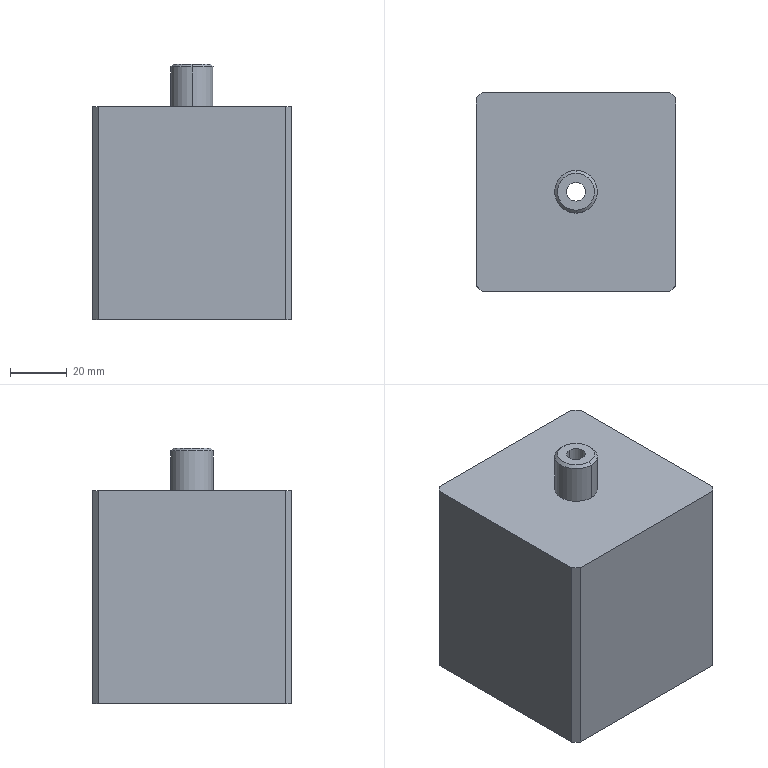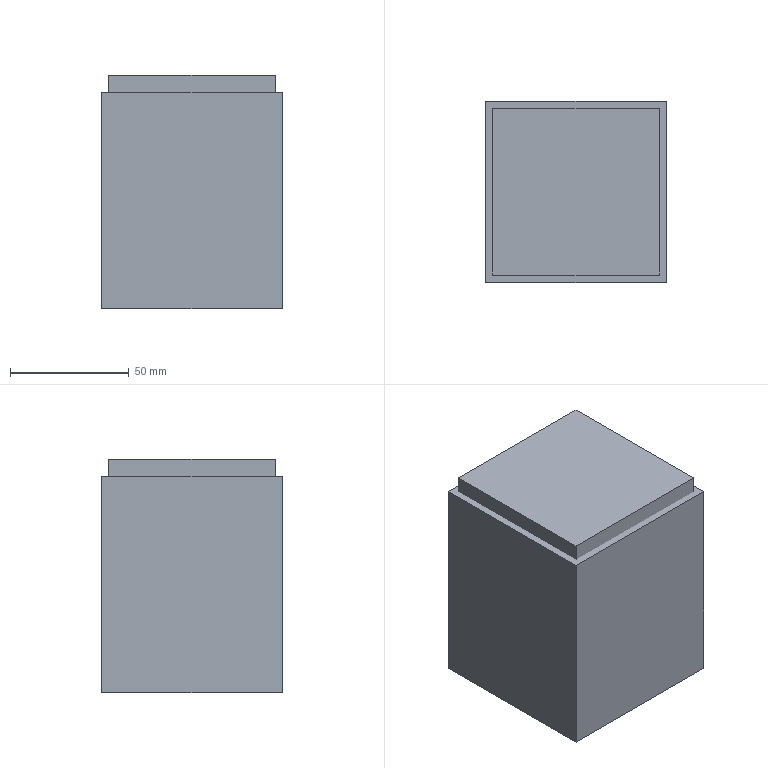CAM job | NX | 3-axis milling, drilling | part box 70 x 70 x 90 mm | stock box 76 x 76 x 98 mm
Tools:
number,name,description,diameter,corner_radius,flute_length,length,flutes
1,D63,Milling Tool-5 Parameters,63.0,0.0,50.0,75.0,2
6,D8A45,Milling Tool-5 Parameters,8.0,0.0,50.0,75.0,2
16,6.6ZT,Drilling Tool,6.6,0.0,35.0,50.0,2
22,D16,Milling Tool-5 Parameters,16.0,0.0,50.0,75.0,2
4,D10,Milling Tool-5 Parameters,10.0,0.0,50.0,75.0,2
18,14.0ZT,Milling Tool-5 Parameters,14.0,0.0,50.0,75.0,2
23,D6R3,Milling Tool-5 Parameters,6.0,3.0,50.0,75.0,2
Operations:
program,operation,operation_type,tool,method,geometry_group,spindle_rpm,surface_speed,feed_per_tooth,feed_cut,feed_plunge,cut_length_mm,path_length_mm,cut_time_min,machine_time_min
1,FLOOR_WALL,VolumeBased25DMillingOperation,D63,METHOD,A,6500.0,1286.0,0.1923,2500.0,100.0,479.797,533.797,0.1919,0.1973
1,DRILLING,Operation,D8A45,METHOD,A,5000.0,0.0,0.0,250.0,0.0,6.4,72.8,0.0256,0.0322
1,DRILLING_COPY,Operation,6.6ZT,METHOD,A,2000.0,41.0,0.0625,250.0,0.0,29.983,119.966,0.1199,0.1289
1,ZLEVEL_PROFILE,ZLevelMilling,D16,METHOD,A,7500.0,376.0,0.1667,2500.0,1000.0,29492.274,29639.474,11.824,11.839
1,ZLEVEL_PROFILE_COPY,ZLevelMilling,D16,METHOD,A,7500.0,376.0,0.0567,850.0,1000.0,1685.604,1925.746,1.978,2.002
1,FLOOR_WALL_1,VolumeBased25DMillingOperation,D10,METHOD,A,7500.0,235.0,0.1667,2500.0,1000.0,15089.067,15547.092,6.121,6.167
1,FLOOR_WALL_1_COPY,VolumeBased25DMillingOperation,D10,METHOD,A,7500.0,235.0,0.0667,1000.0,1000.0,1006.102,1316.289,1.006,1.039
1,PLANAR_MILL,PlanarMilling,D8A45,METHOD,A,7500.0,188.0,0.0833,1250.0,100.0,64.266,121.266,0.0514,0.0571
1,PLANAR_MILL_COPY,PlanarMilling,D8A45,METHOD,A,7500.0,188.0,0.0833,1250.0,100.0,297.482,384.482,0.238,0.2467
2,FLOOR_WALL_COPY,VolumeBased25DMillingOperation,D63,METHOD,B,6500.0,1286.0,0.1923,2500.0,100.0,3646.376,5044.66,1.459,1.598
2,ZLEVEL_PROFILE_COPY_1_COPY,ZLevelMilling,D16,METHOD,B,7500.0,376.0,0.1667,2500.0,1000.0,4039.712,4164.762,1.643,1.656
2,ZLEVEL_PROFILE_COPY_1,ZLevelMilling,D16,METHOD,B,7500.0,376.0,0.1667,2500.0,1000.0,7113.456,7238.506,2.873,2.885
2,ZLEVEL_PROFILE_COPY_COPY,ZLevelMilling,D10,METHOD,B,7500.0,376.0,0.0567,850.0,1000.0,923.803,1117.564,1.082,1.101
2,FLOOR_WALL_1_COPY_COPY,VolumeBased25DMillingOperation,D10,METHOD,B,7500.0,235.0,0.0667,1000.0,1000.0,376.155,569.155,0.3762,0.3955
2,PLANAR_MILL_COPY_COPY,PlanarMilling,D8A45,METHOD,B,7500.0,188.0,0.0833,1250.0,100.0,297.482,354.482,0.238,0.2437
2,DRILLING_COPY_1,Operation,14.0ZT,METHOD,B,3000.0,131.0,0.0417,250.0,0.0,9.4,214.8,0.0376,0.0581
2,ZLEVEL_PROFILE_COPY_1_COPY_COPY,ZLevelMilling,D6R3,METHOD,B,7500.0,376.0,0.1667,2500.0,1000.0,11364.297,11426.497,4.562,4.568